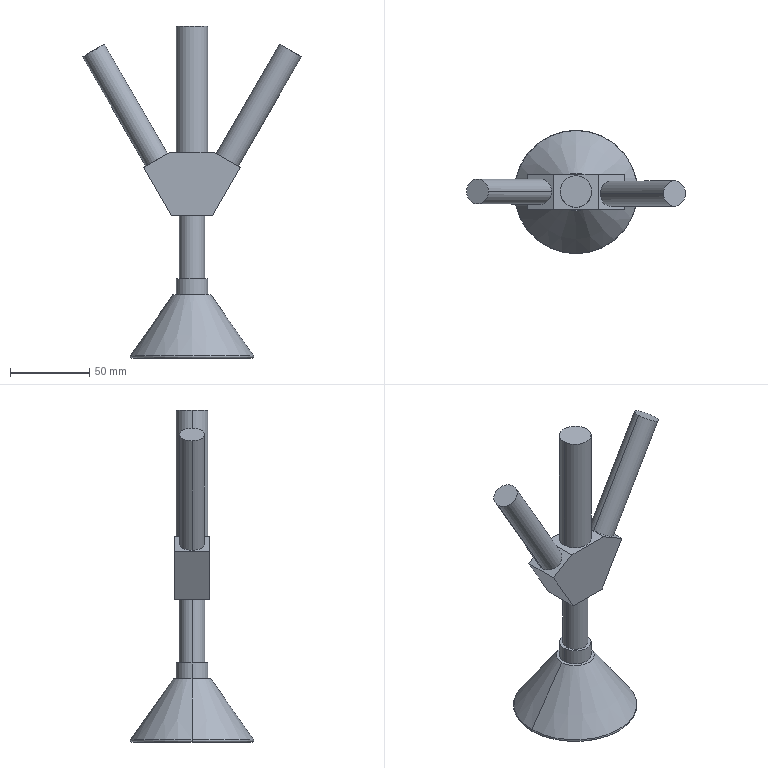Part | NX | features BREP 1 | 1 solid | 31 faces | box 138.349 x 78.158 x 210 mm | volume 141471 mm3 | plane 15 | cylinder 10 | cone 4 | torus 2 | commonest cylinder face diameters 16 x4 20 x4 15.837 x2
STEP:
#1=CARTESIAN_POINT('',(10.,0.,210.));
#2=VERTEX_POINT('',#1);
#3=CARTESIAN_POINT('',(-10.,0.,210.));
#4=VERTEX_POINT('',#3);
#5=CARTESIAN_POINT('',(0.,0.,210.));
#6=DIRECTION('',(0.,0.,1.));
#7=DIRECTION('',(1.,0.,0.));
#8=AXIS2_PLACEMENT_3D('',#5,#6,#7);
#9=CIRCLE('',#8,10.);
#10=EDGE_CURVE('',#2,#4,#9,.T.);
#11=ORIENTED_EDGE('',*,*,#10,.F.);
#12=CARTESIAN_POINT('',(10.,0.,130.));
#13=VERTEX_POINT('',#12);
#14=CARTESIAN_POINT('',(10.,0.,210.));
#15=DIRECTION('',(0.,0.,-1.));
#16=VECTOR('',#15,1000.);
#17=LINE('',#14,#16);
#18=EDGE_CURVE('',#2,#13,#17,.T.);
#19=ORIENTED_EDGE('',*,*,#18,.T.);
#20=CARTESIAN_POINT('',(-10.,0.,130.));
#21=VERTEX_POINT('',#20);
#22=CARTESIAN_POINT('',(0.,0.,130.));
#23=DIRECTION('',(0.,0.,1.));
#24=DIRECTION('',(1.,0.,0.));
#25=AXIS2_PLACEMENT_3D('',#22,#23,#24);
#26=CIRCLE('',#25,10.);
#27=EDGE_CURVE('',#13,#21,#26,.T.);
#28=ORIENTED_EDGE('',*,*,#27,.T.);
#29=CARTESIAN_POINT('',(-10.,0.,210.));
#30=DIRECTION('',(0.,0.,-1.));
#31=VECTOR('',#30,1000.);
#32=LINE('',#29,#31);
#33=EDGE_CURVE('',#4,#21,#32,.T.);
#34=ORIENTED_EDGE('',*,*,#33,.F.);
#35=EDGE_LOOP('',(#11,#19,#28,#34));
#36=FACE_BOUND('',#35,.T.);
#37=CARTESIAN_POINT('',(0.,0.,210.));
#38=DIRECTION('',(0.,0.,-1.));
#39=DIRECTION('',(-1.,0.,0.));
#40=AXIS2_PLACEMENT_3D('',#37,#38,#39);
#41=CYLINDRICAL_SURFACE('',#40,10.);
#42=ADVANCED_FACE('',(#36),#41,.T.);
#43=CARTESIAN_POINT('',(69.21,-1.268,190.503));
#44=VERTEX_POINT('',#43);
#45=CARTESIAN_POINT('',(55.353,-1.268,198.503));
#46=VERTEX_POINT('',#45);
#47=CARTESIAN_POINT('',(62.282,-1.268,194.503));
#48=DIRECTION('',(0.5,0.,0.866));
#49=DIRECTION('',(0.866,0.,-0.5));
#50=AXIS2_PLACEMENT_3D('',#47,#48,#49);
#51=CIRCLE('',#50,8.);
#52=EDGE_CURVE('',#44,#46,#51,.T.);
#53=ORIENTED_EDGE('',*,*,#52,.F.);
#54=CARTESIAN_POINT('',(29.21,-1.268,121.221));
#55=VERTEX_POINT('',#54);
#56=CARTESIAN_POINT('',(69.21,-1.268,190.503));
#57=DIRECTION('',(-0.5,0.,-0.866));
#58=VECTOR('',#57,1000.);
#59=LINE('',#56,#58);
#60=EDGE_CURVE('',#44,#55,#59,.T.);
#61=ORIENTED_EDGE('',*,*,#60,.T.);
#62=CARTESIAN_POINT('',(15.353,-1.268,129.221));
#63=VERTEX_POINT('',#62);
#64=CARTESIAN_POINT('',(22.282,-1.268,125.221));
#65=DIRECTION('',(0.5,0.,0.866));
#66=DIRECTION('',(0.866,0.,-0.5));
#67=AXIS2_PLACEMENT_3D('',#64,#65,#66);
#68=CIRCLE('',#67,8.);
#69=EDGE_CURVE('',#55,#63,#68,.T.);
#70=ORIENTED_EDGE('',*,*,#69,.T.);
#71=CARTESIAN_POINT('',(55.353,-1.268,198.503));
#72=DIRECTION('',(-0.5,0.,-0.866));
#73=VECTOR('',#72,1000.);
#74=LINE('',#71,#73);
#75=EDGE_CURVE('',#46,#63,#74,.T.);
#76=ORIENTED_EDGE('',*,*,#75,.F.);
#77=EDGE_LOOP('',(#53,#61,#70,#76));
#78=FACE_BOUND('',#77,.T.);
#79=CARTESIAN_POINT('',(62.282,-1.268,194.503));
#80=DIRECTION('',(-0.5,0.,-0.866));
#81=DIRECTION('',(-0.866,0.,0.5));
#82=AXIS2_PLACEMENT_3D('',#79,#80,#81);
#83=CYLINDRICAL_SURFACE('',#82,8.);
#84=ADVANCED_FACE('',(#78),#83,.T.);
#85=CARTESIAN_POINT('',(-55.424,0.,198.462));
#86=VERTEX_POINT('',#85);
#87=CARTESIAN_POINT('',(-69.139,0.,190.544));
#88=VERTEX_POINT('',#87);
#89=CARTESIAN_POINT('',(-62.282,0.,194.503));
#90=DIRECTION('',(-0.5,0.,0.866));
#91=DIRECTION('',(0.866,0.,0.5));
#92=AXIS2_PLACEMENT_3D('',#89,#90,#91);
#93=CIRCLE('',#92,7.918);
#94=EDGE_CURVE('',#86,#88,#93,.T.);
#95=ORIENTED_EDGE('',*,*,#94,.F.);
#96=CARTESIAN_POINT('',(-15.424,0.,129.18));
#97=VERTEX_POINT('',#96);
#98=CARTESIAN_POINT('',(-55.424,0.,198.462));
#99=DIRECTION('',(0.5,0.,-0.866));
#100=VECTOR('',#99,1000.);
#101=LINE('',#98,#100);
#102=EDGE_CURVE('',#86,#97,#101,.T.);
#103=ORIENTED_EDGE('',*,*,#102,.T.);
#104=CARTESIAN_POINT('',(-29.139,0.,121.262));
#105=VERTEX_POINT('',#104);
#106=CARTESIAN_POINT('',(-22.282,0.,125.221));
#107=DIRECTION('',(-0.5,0.,0.866));
#108=DIRECTION('',(0.866,0.,0.5));
#109=AXIS2_PLACEMENT_3D('',#106,#107,#108);
#110=CIRCLE('',#109,7.918);
#111=EDGE_CURVE('',#97,#105,#110,.T.);
#112=ORIENTED_EDGE('',*,*,#111,.T.);
#113=CARTESIAN_POINT('',(-69.139,0.,190.544));
#114=DIRECTION('',(0.5,0.,-0.866));
#115=VECTOR('',#114,1000.);
#116=LINE('',#113,#115);
#117=EDGE_CURVE('',#88,#105,#116,.T.);
#118=ORIENTED_EDGE('',*,*,#117,.F.);
#119=EDGE_LOOP('',(#95,#103,#112,#118));
#120=FACE_BOUND('',#119,.T.);
#121=CARTESIAN_POINT('',(-62.282,0.,194.503));
#122=DIRECTION('',(0.5,0.,-0.866));
#123=DIRECTION('',(-0.866,0.,-0.5));
#124=AXIS2_PLACEMENT_3D('',#121,#122,#123);
#125=CYLINDRICAL_SURFACE('',#124,7.918);
#126=ADVANCED_FACE('',(#120),#125,.T.);
#127=CARTESIAN_POINT('',(8.,0.,90.));
#128=VERTEX_POINT('',#127);
#129=CARTESIAN_POINT('',(-8.,0.,90.));
#130=VERTEX_POINT('',#129);
#131=CARTESIAN_POINT('',(0.,0.,90.));
#132=DIRECTION('',(0.,0.,1.));
#133=DIRECTION('',(1.,0.,0.));
#134=AXIS2_PLACEMENT_3D('',#131,#132,#133);
#135=CIRCLE('',#134,8.);
#136=EDGE_CURVE('',#128,#130,#135,.T.);
#137=ORIENTED_EDGE('',*,*,#136,.F.);
#138=CARTESIAN_POINT('',(8.,0.,50.));
#139=VERTEX_POINT('',#138);
#140=CARTESIAN_POINT('',(8.,0.,90.));
#141=DIRECTION('',(0.,0.,-1.));
#142=VECTOR('',#141,1000.);
#143=LINE('',#140,#142);
#144=EDGE_CURVE('',#128,#139,#143,.T.);
#145=ORIENTED_EDGE('',*,*,#144,.T.);
#146=CARTESIAN_POINT('',(-8.,0.,50.));
#147=VERTEX_POINT('',#146);
#148=CARTESIAN_POINT('',(0.,0.,50.));
#149=DIRECTION('',(0.,0.,1.));
#150=DIRECTION('',(1.,0.,0.));
#151=AXIS2_PLACEMENT_3D('',#148,#149,#150);
#152=CIRCLE('',#151,8.);
#153=EDGE_CURVE('',#139,#147,#152,.T.);
#154=ORIENTED_EDGE('',*,*,#153,.T.);
#155=CARTESIAN_POINT('',(-8.,0.,90.));
#156=DIRECTION('',(0.,0.,-1.));
#157=VECTOR('',#156,1000.);
#158=LINE('',#155,#157);
#159=EDGE_CURVE('',#130,#147,#158,.T.);
#160=ORIENTED_EDGE('',*,*,#159,.F.);
#161=EDGE_LOOP('',(#137,#145,#154,#160));
#162=FACE_BOUND('',#161,.T.);
#163=CARTESIAN_POINT('',(0.,0.,90.));
#164=DIRECTION('',(0.,0.,-1.));
#165=DIRECTION('',(-1.,0.,0.));
#166=AXIS2_PLACEMENT_3D('',#163,#164,#165);
#167=CYLINDRICAL_SURFACE('',#166,8.);
#168=ADVANCED_FACE('',(#162),#167,.T.);
#169=CARTESIAN_POINT('',(10.,0.,50.));
#170=VERTEX_POINT('',#169);
#171=CARTESIAN_POINT('',(-10.,0.,50.));
#172=VERTEX_POINT('',#171);
#173=CARTESIAN_POINT('',(0.,0.,50.));
#174=DIRECTION('',(0.,0.,1.));
#175=DIRECTION('',(1.,0.,0.));
#176=AXIS2_PLACEMENT_3D('',#173,#174,#175);
#177=CIRCLE('',#176,10.);
#178=EDGE_CURVE('',#170,#172,#177,.T.);
#179=ORIENTED_EDGE('',*,*,#178,.F.);
#180=CARTESIAN_POINT('',(10.,0.,40.));
#181=VERTEX_POINT('',#180);
#182=CARTESIAN_POINT('',(10.,0.,50.));
#183=DIRECTION('',(0.,0.,-1.));
#184=VECTOR('',#183,1000.);
#185=LINE('',#182,#184);
#186=EDGE_CURVE('',#170,#181,#185,.T.);
#187=ORIENTED_EDGE('',*,*,#186,.T.);
#188=CARTESIAN_POINT('',(-10.,0.,40.));
#189=VERTEX_POINT('',#188);
#190=CARTESIAN_POINT('',(0.,0.,40.));
#191=DIRECTION('',(0.,0.,1.));
#192=DIRECTION('',(1.,0.,0.));
#193=AXIS2_PLACEMENT_3D('',#190,#191,#192);
#194=CIRCLE('',#193,10.);
#195=EDGE_CURVE('',#181,#189,#194,.T.);
#196=ORIENTED_EDGE('',*,*,#195,.T.);
#197=CARTESIAN_POINT('',(-10.,0.,50.));
#198=DIRECTION('',(0.,0.,-1.));
#199=VECTOR('',#198,1000.);
#200=LINE('',#197,#199);
#201=EDGE_CURVE('',#172,#189,#200,.T.);
#202=ORIENTED_EDGE('',*,*,#201,.F.);
#203=EDGE_LOOP('',(#179,#187,#196,#202));
#204=FACE_BOUND('',#203,.T.);
#205=CARTESIAN_POINT('',(0.,0.,50.));
#206=DIRECTION('',(0.,0.,-1.));
#207=DIRECTION('',(-1.,0.,0.));
#208=AXIS2_PLACEMENT_3D('',#205,#206,#207);
#209=CYLINDRICAL_SURFACE('',#208,10.);
#210=ADVANCED_FACE('',(#204),#209,.T.);
#211=CARTESIAN_POINT('',(-38.079,0.,0.));
#212=VERTEX_POINT('',#211);
#213=CARTESIAN_POINT('',(38.079,0.,0.));
#214=VERTEX_POINT('',#213);
#215=CARTESIAN_POINT('',(0.,0.,0.));
#216=DIRECTION('',(0.,0.,-1.));
#217=DIRECTION('',(1.,0.,0.));
#218=AXIS2_PLACEMENT_3D('',#215,#216,#217);
#219=CIRCLE('',#218,38.079);
#220=EDGE_CURVE('',#212,#214,#219,.T.);
#221=ORIENTED_EDGE('',*,*,#220,.F.);
#222=CARTESIAN_POINT('',(-38.898,0.,1.574));
#223=VERTEX_POINT('',#222);
#224=CARTESIAN_POINT('',(-38.079,0.,1.));
#225=DIRECTION('',(0.,1.,0.));
#226=DIRECTION('',(-1.,0.,0.));
#227=AXIS2_PLACEMENT_3D('',#224,#225,#226);
#228=CIRCLE('',#227,1.);
#229=EDGE_CURVE('',#223,#212,#228,.F.);
#230=ORIENTED_EDGE('',*,*,#229,.F.);
#231=CARTESIAN_POINT('',(38.898,0.,1.574));
#232=VERTEX_POINT('',#231);
#233=CARTESIAN_POINT('',(0.,0.,1.574));
#234=DIRECTION('',(0.,0.,1.));
#235=DIRECTION('',(1.,0.,0.));
#236=AXIS2_PLACEMENT_3D('',#233,#234,#235);
#237=CIRCLE('',#236,38.898);
#238=EDGE_CURVE('',#232,#223,#237,.T.);
#239=ORIENTED_EDGE('',*,*,#238,.F.);
#240=CARTESIAN_POINT('',(38.079,0.,1.));
#241=DIRECTION('',(0.,-1.,0.));
#242=DIRECTION('',(0.,0.,-1.));
#243=AXIS2_PLACEMENT_3D('',#240,#241,#242);
#244=CIRCLE('',#243,1.);
#245=EDGE_CURVE('',#232,#214,#244,.F.);
#246=ORIENTED_EDGE('',*,*,#245,.T.);
#247=EDGE_LOOP('',(#221,#230,#239,#246));
#248=FACE_BOUND('',#247,.T.);
#249=CARTESIAN_POINT('',(0.,0.,1.));
#250=DIRECTION('',(0.,0.,1.));
#251=DIRECTION('',(1.,0.,0.));
#252=AXIS2_PLACEMENT_3D('',#249,#250,#251);
#253=TOROIDAL_SURFACE('',#252,38.079,1.);
#254=ADVANCED_FACE('',(#248),#253,.T.);
#255=CARTESIAN_POINT('',(5.992,0.,40.));
#256=VERTEX_POINT('',#255);
#257=CARTESIAN_POINT('',(-5.992,0.,40.));
#258=VERTEX_POINT('',#257);
#259=CARTESIAN_POINT('',(0.,0.,40.));
#260=DIRECTION('',(0.,0.,-1.));
#261=DIRECTION('',(-1.,0.,0.));
#262=AXIS2_PLACEMENT_3D('',#259,#260,#261);
#263=CIRCLE('',#262,5.992);
#264=EDGE_CURVE('',#256,#258,#263,.T.);
#265=ORIENTED_EDGE('',*,*,#264,.F.);
#266=CARTESIAN_POINT('',(34.,0.,0.));
#267=VERTEX_POINT('',#266);
#268=CARTESIAN_POINT('',(34.,0.,0.));
#269=DIRECTION('',(0.5736,0.,-0.8192));
#270=VECTOR('',#269,1000.);
#271=LINE('',#268,#270);
#272=EDGE_CURVE('',#256,#267,#271,.T.);
#273=ORIENTED_EDGE('',*,*,#272,.T.);
#274=CARTESIAN_POINT('',(-34.,0.,0.));
#275=VERTEX_POINT('',#274);
#276=CARTESIAN_POINT('',(0.,0.,0.));
#277=DIRECTION('',(0.,0.,-1.));
#278=DIRECTION('',(-1.,0.,0.));
#279=AXIS2_PLACEMENT_3D('',#276,#277,#278);
#280=CIRCLE('',#279,34.);
#281=EDGE_CURVE('',#267,#275,#280,.T.);
#282=ORIENTED_EDGE('',*,*,#281,.T.);
#283=CARTESIAN_POINT('',(-34.,0.,0.));
#284=DIRECTION('',(-0.5736,0.,-0.8192));
#285=VECTOR('',#284,1000.);
#286=LINE('',#283,#285);
#287=EDGE_CURVE('',#258,#275,#286,.T.);
#288=ORIENTED_EDGE('',*,*,#287,.F.);
#289=EDGE_LOOP('',(#265,#273,#282,#288));
#290=FACE_BOUND('',#289,.T.);
#291=CARTESIAN_POINT('',(0.,0.,0.));
#292=DIRECTION('',(0.,0.,-1.));
#293=DIRECTION('',(-1.,0.,0.));
#294=AXIS2_PLACEMENT_3D('',#291,#292,#293);
#295=CONICAL_SURFACE('',#294,34.,0.6109);
#296=ADVANCED_FACE('',(#290),#295,.F.);
#297=CARTESIAN_POINT('',(-11.992,0.,40.));
#298=VERTEX_POINT('',#297);
#299=CARTESIAN_POINT('',(11.992,0.,40.));
#300=VERTEX_POINT('',#299);
#301=CARTESIAN_POINT('',(0.,0.,40.));
#302=DIRECTION('',(0.,0.,1.));
#303=DIRECTION('',(1.,0.,0.));
#304=AXIS2_PLACEMENT_3D('',#301,#302,#303);
#305=CIRCLE('',#304,11.992);
#306=EDGE_CURVE('',#298,#300,#305,.T.);
#307=ORIENTED_EDGE('',*,*,#306,.F.);
#308=CARTESIAN_POINT('',(-40.,0.,0.));
#309=DIRECTION('',(-0.5736,0.,-0.8192));
#310=VECTOR('',#309,1000.);
#311=LINE('',#308,#310);
#312=EDGE_CURVE('',#223,#298,#311,.F.);
#313=ORIENTED_EDGE('',*,*,#312,.F.);
#314=CARTESIAN_POINT('',(0.,0.,1.574));
#315=DIRECTION('',(0.,0.,1.));
#316=DIRECTION('',(1.,0.,0.));
#317=AXIS2_PLACEMENT_3D('',#314,#315,#316);
#318=CIRCLE('',#317,38.898);
#319=EDGE_CURVE('',#223,#232,#318,.T.);
#320=ORIENTED_EDGE('',*,*,#319,.T.);
#321=CARTESIAN_POINT('',(40.,0.,0.));
#322=DIRECTION('',(0.5736,0.,-0.8192));
#323=VECTOR('',#322,1000.);
#324=LINE('',#321,#323);
#325=EDGE_CURVE('',#232,#300,#324,.F.);
#326=ORIENTED_EDGE('',*,*,#325,.T.);
#327=EDGE_LOOP('',(#307,#313,#320,#326));
#328=FACE_BOUND('',#327,.T.);
#329=CARTESIAN_POINT('',(0.,0.,0.));
#330=DIRECTION('',(0.,0.,-1.));
#331=DIRECTION('',(1.,0.,0.));
#332=AXIS2_PLACEMENT_3D('',#329,#330,#331);
#333=CONICAL_SURFACE('',#332,40.,0.6109);
#334=ADVANCED_FACE('',(#328),#333,.T.);
#335=ORIENTED_EDGE('',*,*,#312,.T.);
#336=CARTESIAN_POINT('',(0.,0.,40.));
#337=DIRECTION('',(0.,0.,1.));
#338=DIRECTION('',(1.,0.,0.));
#339=AXIS2_PLACEMENT_3D('',#336,#337,#338);
#340=CIRCLE('',#339,11.992);
#341=EDGE_CURVE('',#300,#298,#340,.T.);
#342=ORIENTED_EDGE('',*,*,#341,.F.);
#343=ORIENTED_EDGE('',*,*,#325,.F.);
#344=ORIENTED_EDGE('',*,*,#238,.T.);
#345=EDGE_LOOP('',(#335,#342,#343,#344));
#346=FACE_BOUND('',#345,.T.);
#347=CARTESIAN_POINT('',(0.,0.,0.));
#348=DIRECTION('',(0.,0.,-1.));
#349=DIRECTION('',(1.,0.,0.));
#350=AXIS2_PLACEMENT_3D('',#347,#348,#349);
#351=CONICAL_SURFACE('',#350,40.,0.6109);
#352=ADVANCED_FACE('',(#346),#351,.T.);
#353=ORIENTED_EDGE('',*,*,#341,.T.);
#354=ORIENTED_EDGE('',*,*,#306,.T.);
#355=EDGE_LOOP('',(#353,#354));
#356=FACE_BOUND('',#355,.T.);
#357=CARTESIAN_POINT('',(0.,0.,40.));
#358=DIRECTION('',(0.,0.,1.));
#359=DIRECTION('',(1.,0.,0.));
#360=AXIS2_PLACEMENT_3D('',#357,#358,#359);
#361=CIRCLE('',#360,10.);
#362=EDGE_CURVE('',#189,#181,#361,.T.);
#363=ORIENTED_EDGE('',*,*,#362,.F.);
#364=ORIENTED_EDGE('',*,*,#195,.F.);
#365=EDGE_LOOP('',(#363,#364));
#366=FACE_BOUND('',#365,.T.);
#367=CARTESIAN_POINT('',(0.,0.,40.));
#368=DIRECTION('',(0.,0.,1.));
#369=DIRECTION('',(1.,0.,0.));
#370=AXIS2_PLACEMENT_3D('',#367,#368,#369);
#371=PLANE('',#370);
#372=ADVANCED_FACE('',(#356,#366),#371,.T.);
#373=CARTESIAN_POINT('',(0.,0.,0.));
#374=DIRECTION('',(0.,0.,-1.));
#375=DIRECTION('',(1.,0.,0.));
#376=AXIS2_PLACEMENT_3D('',#373,#374,#375);
#377=CIRCLE('',#376,38.079);
#378=EDGE_CURVE('',#214,#212,#377,.T.);
#379=ORIENTED_EDGE('',*,*,#378,.T.);
#380=ORIENTED_EDGE('',*,*,#220,.T.);
#381=EDGE_LOOP('',(#379,#380));
#382=FACE_BOUND('',#381,.T.);
#383=CARTESIAN_POINT('',(0.,0.,0.));
#384=DIRECTION('',(0.,0.,-1.));
#385=DIRECTION('',(-1.,0.,0.));
#386=AXIS2_PLACEMENT_3D('',#383,#384,#385);
#387=CIRCLE('',#386,34.);
#388=EDGE_CURVE('',#275,#267,#387,.T.);
#389=ORIENTED_EDGE('',*,*,#388,.F.);
#390=ORIENTED_EDGE('',*,*,#281,.F.);
#391=EDGE_LOOP('',(#389,#390));
#392=FACE_BOUND('',#391,.T.);
#393=CARTESIAN_POINT('',(0.,0.,0.));
#394=DIRECTION('',(0.,0.,1.));
#395=DIRECTION('',(1.,0.,0.));
#396=AXIS2_PLACEMENT_3D('',#393,#394,#395);
#397=PLANE('',#396);
#398=ADVANCED_FACE('',(#382,#392),#397,.F.);
#399=ORIENTED_EDGE('',*,*,#272,.F.);
#400=CARTESIAN_POINT('',(0.,0.,40.));
#401=DIRECTION('',(0.,0.,-1.));
#402=DIRECTION('',(-1.,0.,0.));
#403=AXIS2_PLACEMENT_3D('',#400,#401,#402);
#404=CIRCLE('',#403,5.992);
#405=EDGE_CURVE('',#258,#256,#404,.T.);
#406=ORIENTED_EDGE('',*,*,#405,.F.);
#407=ORIENTED_EDGE('',*,*,#287,.T.);
#408=ORIENTED_EDGE('',*,*,#388,.T.);
#409=EDGE_LOOP('',(#399,#406,#407,#408));
#410=FACE_BOUND('',#409,.T.);
#411=CARTESIAN_POINT('',(0.,0.,0.));
#412=DIRECTION('',(0.,0.,-1.));
#413=DIRECTION('',(-1.,0.,0.));
#414=AXIS2_PLACEMENT_3D('',#411,#412,#413);
#415=CONICAL_SURFACE('',#414,34.,0.6109);
#416=ADVANCED_FACE('',(#410),#415,.F.);
#417=ORIENTED_EDGE('',*,*,#229,.T.);
#418=ORIENTED_EDGE('',*,*,#378,.F.);
#419=ORIENTED_EDGE('',*,*,#245,.F.);
#420=ORIENTED_EDGE('',*,*,#319,.F.);
#421=EDGE_LOOP('',(#417,#418,#419,#420));
#422=FACE_BOUND('',#421,.T.);
#423=CARTESIAN_POINT('',(0.,0.,1.));
#424=DIRECTION('',(0.,0.,1.));
#425=DIRECTION('',(1.,0.,0.));
#426=AXIS2_PLACEMENT_3D('',#423,#424,#425);
#427=TOROIDAL_SURFACE('',#426,38.079,1.);
#428=ADVANCED_FACE('',(#422),#427,.T.);
#429=CARTESIAN_POINT('',(0.,0.,50.));
#430=DIRECTION('',(0.,0.,1.));
#431=DIRECTION('',(1.,0.,0.));
#432=AXIS2_PLACEMENT_3D('',#429,#430,#431);
#433=CIRCLE('',#432,10.);
#434=EDGE_CURVE('',#172,#170,#433,.T.);
#435=ORIENTED_EDGE('',*,*,#434,.T.);
#436=ORIENTED_EDGE('',*,*,#178,.T.);
#437=EDGE_LOOP('',(#435,#436));
#438=FACE_BOUND('',#437,.T.);
#439=CARTESIAN_POINT('',(0.,0.,50.));
#440=DIRECTION('',(0.,0.,1.));
#441=DIRECTION('',(1.,0.,0.));
#442=AXIS2_PLACEMENT_3D('',#439,#440,#441);
#443=CIRCLE('',#442,8.);
#444=EDGE_CURVE('',#147,#139,#443,.T.);
#445=ORIENTED_EDGE('',*,*,#444,.F.);
#446=ORIENTED_EDGE('',*,*,#153,.F.);
#447=EDGE_LOOP('',(#445,#446));
#448=FACE_BOUND('',#447,.T.);
#449=CARTESIAN_POINT('',(0.,0.,50.));
#450=DIRECTION('',(0.,0.,1.));
#451=DIRECTION('',(1.,0.,0.));
#452=AXIS2_PLACEMENT_3D('',#449,#450,#451);
#453=PLANE('',#452);
#454=ADVANCED_FACE('',(#438,#448),#453,.T.);
#455=ORIENTED_EDGE('',*,*,#186,.F.);
#456=ORIENTED_EDGE('',*,*,#434,.F.);
#457=ORIENTED_EDGE('',*,*,#201,.T.);
#458=ORIENTED_EDGE('',*,*,#362,.T.);
#459=EDGE_LOOP('',(#455,#456,#457,#458));
#460=FACE_BOUND('',#459,.T.);
#461=CARTESIAN_POINT('',(0.,0.,50.));
#462=DIRECTION('',(0.,0.,-1.));
#463=DIRECTION('',(-1.,0.,0.));
#464=AXIS2_PLACEMENT_3D('',#461,#462,#463);
#465=CYLINDRICAL_SURFACE('',#464,10.);
#466=ADVANCED_FACE('',(#460),#465,.T.);
#467=ORIENTED_EDGE('',*,*,#405,.T.);
#468=ORIENTED_EDGE('',*,*,#264,.T.);
#469=EDGE_LOOP('',(#467,#468));
#470=FACE_BOUND('',#469,.T.);
#471=CARTESIAN_POINT('',(0.,0.,40.));
#472=DIRECTION('',(0.,0.,1.));
#473=DIRECTION('',(1.,0.,0.));
#474=AXIS2_PLACEMENT_3D('',#471,#472,#473);
#475=PLANE('',#474);
#476=ADVANCED_FACE('',(#470),#475,.F.);
#477=ORIENTED_EDGE('',*,*,#144,.F.);
#478=CARTESIAN_POINT('',(0.,0.,90.));
#479=DIRECTION('',(0.,0.,1.));
#480=DIRECTION('',(1.,0.,0.));
#481=AXIS2_PLACEMENT_3D('',#478,#479,#480);
#482=CIRCLE('',#481,8.);
#483=EDGE_CURVE('',#130,#128,#482,.T.);
#484=ORIENTED_EDGE('',*,*,#483,.F.);
#485=ORIENTED_EDGE('',*,*,#159,.T.);
#486=ORIENTED_EDGE('',*,*,#444,.T.);
#487=EDGE_LOOP('',(#477,#484,#485,#486));
#488=FACE_BOUND('',#487,.T.);
#489=CARTESIAN_POINT('',(0.,0.,90.));
#490=DIRECTION('',(0.,0.,-1.));
#491=DIRECTION('',(-1.,0.,0.));
#492=AXIS2_PLACEMENT_3D('',#489,#490,#491);
#493=CYLINDRICAL_SURFACE('',#492,8.);
#494=ADVANCED_FACE('',(#488),#493,.T.);
#495=CARTESIAN_POINT('',(12.983,11.088,90.));
#496=VERTEX_POINT('',#495);
#497=CARTESIAN_POINT('',(-12.983,11.088,90.));
#498=VERTEX_POINT('',#497);
#499=CARTESIAN_POINT('',(-12.983,11.088,90.));
#500=DIRECTION('',(-1.,0.,0.));
#501=VECTOR('',#500,1000.);
#502=LINE('',#499,#501);
#503=EDGE_CURVE('',#496,#498,#502,.T.);
#504=ORIENTED_EDGE('',*,*,#503,.T.);
#505=CARTESIAN_POINT('',(-30.559,11.088,120.442));
#506=VERTEX_POINT('',#505);
#507=CARTESIAN_POINT('',(-12.983,11.088,90.));
#508=DIRECTION('',(-0.5,0.,0.866));
#509=VECTOR('',#508,1000.);
#510=LINE('',#507,#509);
#511=EDGE_CURVE('',#498,#506,#510,.T.);
#512=ORIENTED_EDGE('',*,*,#511,.T.);
#513=CARTESIAN_POINT('',(-14.004,11.088,130.));
#514=VERTEX_POINT('',#513);
#515=CARTESIAN_POINT('',(-30.559,11.088,120.442));
#516=DIRECTION('',(0.866,0.,0.5));
#517=VECTOR('',#516,1000.);
#518=LINE('',#515,#517);
#519=EDGE_CURVE('',#506,#514,#518,.T.);
#520=ORIENTED_EDGE('',*,*,#519,.T.);
#521=CARTESIAN_POINT('',(14.004,11.088,130.));
#522=VERTEX_POINT('',#521);
#523=CARTESIAN_POINT('',(-12.983,11.088,130.));
#524=DIRECTION('',(-1.,0.,0.));
#525=VECTOR('',#524,1000.);
#526=LINE('',#523,#525);
#527=EDGE_CURVE('',#522,#514,#526,.T.);
#528=ORIENTED_EDGE('',*,*,#527,.F.);
#529=CARTESIAN_POINT('',(30.559,11.088,120.442));
#530=VERTEX_POINT('',#529);
#531=CARTESIAN_POINT('',(30.559,11.088,120.442));
#532=DIRECTION('',(0.866,0.,-0.5));
#533=VECTOR('',#532,1000.);
#534=LINE('',#531,#533);
#535=EDGE_CURVE('',#522,#530,#534,.T.);
#536=ORIENTED_EDGE('',*,*,#535,.T.);
#537=CARTESIAN_POINT('',(12.983,11.088,90.));
#538=DIRECTION('',(-0.5,0.,-0.866));
#539=VECTOR('',#538,1000.);
#540=LINE('',#537,#539);
#541=EDGE_CURVE('',#530,#496,#540,.T.);
#542=ORIENTED_EDGE('',*,*,#541,.T.);
#543=EDGE_LOOP('',(#504,#512,#520,#528,#536,#542));
#544=FACE_BOUND('',#543,.T.);
#545=CARTESIAN_POINT('',(-12.983,11.088,130.));
#546=DIRECTION('',(0.,-1.,0.));
#547=DIRECTION('',(0.,0.,-1.));
#548=AXIS2_PLACEMENT_3D('',#545,#546,#547);
#549=PLANE('',#548);
#550=ADVANCED_FACE('',(#544),#549,.F.);
#551=CARTESIAN_POINT('',(-12.983,-11.088,90.));
#552=VERTEX_POINT('',#551);
#553=CARTESIAN_POINT('',(12.983,-11.088,90.));
#554=VERTEX_POINT('',#553);
#555=CARTESIAN_POINT('',(-12.983,-11.088,90.));
#556=DIRECTION('',(1.,0.,0.));
#557=VECTOR('',#556,1000.);
#558=LINE('',#555,#557);
#559=EDGE_CURVE('',#552,#554,#558,.T.);
#560=ORIENTED_EDGE('',*,*,#559,.T.);
#561=CARTESIAN_POINT('',(30.559,-11.088,120.442));
#562=VERTEX_POINT('',#561);
#563=CARTESIAN_POINT('',(12.983,-11.088,90.));
#564=DIRECTION('',(0.5,0.,0.866));
#565=VECTOR('',#564,1000.);
#566=LINE('',#563,#565);
#567=EDGE_CURVE('',#554,#562,#566,.T.);
#568=ORIENTED_EDGE('',*,*,#567,.T.);
#569=CARTESIAN_POINT('',(14.004,-11.088,130.));
#570=VERTEX_POINT('',#569);
#571=CARTESIAN_POINT('',(30.559,-11.088,120.442));
#572=DIRECTION('',(-0.866,0.,0.5));
#573=VECTOR('',#572,1000.);
#574=LINE('',#571,#573);
#575=EDGE_CURVE('',#562,#570,#574,.T.);
#576=ORIENTED_EDGE('',*,*,#575,.T.);
#577=CARTESIAN_POINT('',(-14.004,-11.088,130.));
#578=VERTEX_POINT('',#577);
#579=CARTESIAN_POINT('',(-12.983,-11.088,130.));
#580=DIRECTION('',(1.,0.,0.));
#581=VECTOR('',#580,1000.);
#582=LINE('',#579,#581);
#583=EDGE_CURVE('',#578,#570,#582,.T.);
#584=ORIENTED_EDGE('',*,*,#583,.F.);
#585=CARTESIAN_POINT('',(-30.559,-11.088,120.442));
#586=VERTEX_POINT('',#585);
#587=CARTESIAN_POINT('',(-30.559,-11.088,120.442));
#588=DIRECTION('',(-0.866,0.,-0.5));
#589=VECTOR('',#588,1000.);
#590=LINE('',#587,#589);
#591=EDGE_CURVE('',#578,#586,#590,.T.);
#592=ORIENTED_EDGE('',*,*,#591,.T.);
#593=CARTESIAN_POINT('',(-12.983,-11.088,90.));
#594=DIRECTION('',(0.5,0.,-0.866));
#595=VECTOR('',#594,1000.);
#596=LINE('',#593,#595);
#597=EDGE_CURVE('',#586,#552,#596,.T.);
#598=ORIENTED_EDGE('',*,*,#597,.T.);
#599=EDGE_LOOP('',(#560,#568,#576,#584,#592,#598));
#600=FACE_BOUND('',#599,.T.);
#601=CARTESIAN_POINT('',(-12.983,-11.088,130.));
#602=DIRECTION('',(0.,1.,0.));
#603=DIRECTION('',(1.,0.,0.));
#604=AXIS2_PLACEMENT_3D('',#601,#602,#603);
#605=PLANE('',#604);
#606=ADVANCED_FACE('',(#600),#605,.F.);
#607=ORIENTED_EDGE('',*,*,#583,.T.);
#608=CARTESIAN_POINT('',(14.004,-54.779,130.));
#609=DIRECTION('',(0.,1.,0.));
#610=VECTOR('',#609,1000.);
#611=LINE('',#608,#610);
#612=EDGE_CURVE('',#570,#522,#611,.T.);
#613=ORIENTED_EDGE('',*,*,#612,.T.);
#614=ORIENTED_EDGE('',*,*,#527,.T.);
#615=CARTESIAN_POINT('',(-14.004,-54.779,130.));
#616=DIRECTION('',(0.,1.,0.));
#617=VECTOR('',#616,1000.);
#618=LINE('',#615,#617);
#619=EDGE_CURVE('',#578,#514,#618,.T.);
#620=ORIENTED_EDGE('',*,*,#619,.F.);
#621=EDGE_LOOP('',(#607,#613,#614,#620));
#622=FACE_BOUND('',#621,.T.);
#623=CARTESIAN_POINT('',(0.,0.,130.));
#624=DIRECTION('',(0.,0.,1.));
#625=DIRECTION('',(1.,0.,0.));
#626=AXIS2_PLACEMENT_3D('',#623,#624,#625);
#627=CIRCLE('',#626,10.);
#628=EDGE_CURVE('',#21,#13,#627,.T.);
#629=ORIENTED_EDGE('',*,*,#628,.F.);
#630=ORIENTED_EDGE('',*,*,#27,.F.);
#631=EDGE_LOOP('',(#629,#630));
#632=FACE_BOUND('',#631,.T.);
#633=CARTESIAN_POINT('',(0.,0.,130.));
#634=DIRECTION('',(0.,0.,-1.));
#635=DIRECTION('',(0.,-1.,0.));
#636=AXIS2_PLACEMENT_3D('',#633,#634,#635);
#637=PLANE('',#636);
#638=ADVANCED_FACE('',(#622,#632),#637,.F.);
#639=CARTESIAN_POINT('',(12.983,-11.088,90.));
#640=DIRECTION('',(0.,1.,0.));
#641=VECTOR('',#640,1000.);
#642=LINE('',#639,#641);
#643=EDGE_CURVE('',#554,#496,#642,.T.);
#644=ORIENTED_EDGE('',*,*,#643,.F.);
#645=ORIENTED_EDGE('',*,*,#559,.F.);
#646=CARTESIAN_POINT('',(-12.983,-11.088,90.));
#647=DIRECTION('',(0.,-1.,0.));
#648=VECTOR('',#647,1000.);
#649=LINE('',#646,#648);
#650=EDGE_CURVE('',#498,#552,#649,.T.);
#651=ORIENTED_EDGE('',*,*,#650,.F.);
#652=ORIENTED_EDGE('',*,*,#503,.F.);
#653=EDGE_LOOP('',(#644,#645,#651,#652));
#654=FACE_BOUND('',#653,.T.);
#655=ORIENTED_EDGE('',*,*,#483,.T.);
#656=ORIENTED_EDGE('',*,*,#136,.T.);
#657=EDGE_LOOP('',(#655,#656));
#658=FACE_BOUND('',#657,.T.);
#659=CARTESIAN_POINT('',(0.,0.,90.));
#660=DIRECTION('',(0.,0.,-1.));
#661=DIRECTION('',(0.,-1.,0.));
#662=AXIS2_PLACEMENT_3D('',#659,#660,#661);
#663=PLANE('',#662);
#664=ADVANCED_FACE('',(#654,#658),#663,.T.);
#665=ORIENTED_EDGE('',*,*,#591,.F.);
#666=ORIENTED_EDGE('',*,*,#619,.T.);
#667=ORIENTED_EDGE('',*,*,#519,.F.);
#668=CARTESIAN_POINT('',(-30.559,-54.779,120.442));
#669=DIRECTION('',(0.,1.,0.));
#670=VECTOR('',#669,1000.);
#671=LINE('',#668,#670);
#672=EDGE_CURVE('',#586,#506,#671,.T.);
#673=ORIENTED_EDGE('',*,*,#672,.F.);
#674=EDGE_LOOP('',(#665,#666,#667,#673));
#675=FACE_BOUND('',#674,.T.);
#676=CARTESIAN_POINT('',(-22.282,0.,125.221));
#677=DIRECTION('',(-0.5,0.,0.866));
#678=DIRECTION('',(0.866,0.,0.5));
#679=AXIS2_PLACEMENT_3D('',#676,#677,#678);
#680=CIRCLE('',#679,7.918);
#681=EDGE_CURVE('',#105,#97,#680,.T.);
#682=ORIENTED_EDGE('',*,*,#681,.F.);
#683=ORIENTED_EDGE('',*,*,#111,.F.);
#684=EDGE_LOOP('',(#682,#683));
#685=FACE_BOUND('',#684,.T.);
#686=CARTESIAN_POINT('',(-30.559,-54.779,120.442));
#687=DIRECTION('',(-0.5,0.,0.866));
#688=DIRECTION('',(0.,1.,0.));
#689=AXIS2_PLACEMENT_3D('',#686,#687,#688);
#690=PLANE('',#689);
#691=ADVANCED_FACE('',(#675,#685),#690,.T.);
#692=ORIENTED_EDGE('',*,*,#597,.F.);
#693=ORIENTED_EDGE('',*,*,#672,.T.);
#694=ORIENTED_EDGE('',*,*,#511,.F.);
#695=ORIENTED_EDGE('',*,*,#650,.T.);
#696=EDGE_LOOP('',(#692,#693,#694,#695));
#697=FACE_BOUND('',#696,.T.);
#698=CARTESIAN_POINT('',(-12.983,-54.779,90.));
#699=DIRECTION('',(-0.866,0.,-0.5));
#700=DIRECTION('',(-0.5,0.,0.866));
#701=AXIS2_PLACEMENT_3D('',#698,#699,#700);
#702=PLANE('',#701);
#703=ADVANCED_FACE('',(#697),#702,.T.);
#704=ORIENTED_EDGE('',*,*,#567,.F.);
#705=ORIENTED_EDGE('',*,*,#643,.T.);
#706=ORIENTED_EDGE('',*,*,#541,.F.);
#707=CARTESIAN_POINT('',(30.559,-54.779,120.442));
#708=DIRECTION('',(0.,1.,0.));
#709=VECTOR('',#708,1000.);
#710=LINE('',#707,#709);
#711=EDGE_CURVE('',#562,#530,#710,.T.);
#712=ORIENTED_EDGE('',*,*,#711,.F.);
#713=EDGE_LOOP('',(#704,#705,#706,#712));
#714=FACE_BOUND('',#713,.T.);
#715=CARTESIAN_POINT('',(12.983,-54.779,90.));
#716=DIRECTION('',(0.866,0.,-0.5));
#717=DIRECTION('',(0.,-1.,0.));
#718=AXIS2_PLACEMENT_3D('',#715,#716,#717);
#719=PLANE('',#718);
#720=ADVANCED_FACE('',(#714),#719,.T.);
#721=ORIENTED_EDGE('',*,*,#575,.F.);
#722=ORIENTED_EDGE('',*,*,#711,.T.);
#723=ORIENTED_EDGE('',*,*,#535,.F.);
#724=ORIENTED_EDGE('',*,*,#612,.F.);
#725=EDGE_LOOP('',(#721,#722,#723,#724));
#726=FACE_BOUND('',#725,.T.);
#727=CARTESIAN_POINT('',(22.282,-1.268,125.221));
#728=DIRECTION('',(0.5,0.,0.866));
#729=DIRECTION('',(0.866,0.,-0.5));
#730=AXIS2_PLACEMENT_3D('',#727,#728,#729);
#731=CIRCLE('',#730,8.);
#732=EDGE_CURVE('',#63,#55,#731,.T.);
#733=ORIENTED_EDGE('',*,*,#732,.F.);
#734=ORIENTED_EDGE('',*,*,#69,.F.);
#735=EDGE_LOOP('',(#733,#734));
#736=FACE_BOUND('',#735,.T.);
#737=CARTESIAN_POINT('',(30.559,-54.779,120.442));
#738=DIRECTION('',(0.5,0.,0.866));
#739=DIRECTION('',(0.,-1.,0.));
#740=AXIS2_PLACEMENT_3D('',#737,#738,#739);
#741=PLANE('',#740);
#742=ADVANCED_FACE('',(#726,#736),#741,.T.);
#743=ORIENTED_EDGE('',*,*,#102,.F.);
#744=CARTESIAN_POINT('',(-62.282,0.,194.503));
#745=DIRECTION('',(-0.5,0.,0.866));
#746=DIRECTION('',(0.866,0.,0.5));
#747=AXIS2_PLACEMENT_3D('',#744,#745,#746);
#748=CIRCLE('',#747,7.918);
#749=EDGE_CURVE('',#88,#86,#748,.T.);
#750=ORIENTED_EDGE('',*,*,#749,.F.);
#751=ORIENTED_EDGE('',*,*,#117,.T.);
#752=ORIENTED_EDGE('',*,*,#681,.T.);
#753=EDGE_LOOP('',(#743,#750,#751,#752));
#754=FACE_BOUND('',#753,.T.);
#755=CARTESIAN_POINT('',(-62.282,0.,194.503));
#756=DIRECTION('',(0.5,0.,-0.866));
#757=DIRECTION('',(-0.866,0.,-0.5));
#758=AXIS2_PLACEMENT_3D('',#755,#756,#757);
#759=CYLINDRICAL_SURFACE('',#758,7.918);
#760=ADVANCED_FACE('',(#754),#759,.T.);
#761=ORIENTED_EDGE('',*,*,#749,.T.);
#762=ORIENTED_EDGE('',*,*,#94,.T.);
#763=EDGE_LOOP('',(#761,#762));
#764=FACE_BOUND('',#763,.T.);
#765=CARTESIAN_POINT('',(-62.282,0.,194.503));
#766=DIRECTION('',(-0.5,0.,0.866));
#767=DIRECTION('',(0.,1.,0.));
#768=AXIS2_PLACEMENT_3D('',#765,#766,#767);
#769=PLANE('',#768);
#770=ADVANCED_FACE('',(#764),#769,.T.);
#771=ORIENTED_EDGE('',*,*,#60,.F.);
#772=CARTESIAN_POINT('',(62.282,-1.268,194.503));
#773=DIRECTION('',(0.5,0.,0.866));
#774=DIRECTION('',(0.866,0.,-0.5));
#775=AXIS2_PLACEMENT_3D('',#772,#773,#774);
#776=CIRCLE('',#775,8.);
#777=EDGE_CURVE('',#46,#44,#776,.T.);
#778=ORIENTED_EDGE('',*,*,#777,.F.);
#779=ORIENTED_EDGE('',*,*,#75,.T.);
#780=ORIENTED_EDGE('',*,*,#732,.T.);
#781=EDGE_LOOP('',(#771,#778,#779,#780));
#782=FACE_BOUND('',#781,.T.);
#783=CARTESIAN_POINT('',(62.282,-1.268,194.503));
#784=DIRECTION('',(-0.5,0.,-0.866));
#785=DIRECTION('',(-0.866,0.,0.5));
#786=AXIS2_PLACEMENT_3D('',#783,#784,#785);
#787=CYLINDRICAL_SURFACE('',#786,8.);
#788=ADVANCED_FACE('',(#782),#787,.T.);
#789=ORIENTED_EDGE('',*,*,#777,.T.);
#790=ORIENTED_EDGE('',*,*,#52,.T.);
#791=EDGE_LOOP('',(#789,#790));
#792=FACE_BOUND('',#791,.T.);
#793=CARTESIAN_POINT('',(62.282,-1.268,194.503));
#794=DIRECTION('',(0.5,0.,0.866));
#795=DIRECTION('',(0.,-1.,0.));
#796=AXIS2_PLACEMENT_3D('',#793,#794,#795);
#797=PLANE('',#796);
#798=ADVANCED_FACE('',(#792),#797,.T.);
#799=ORIENTED_EDGE('',*,*,#18,.F.);
#800=CARTESIAN_POINT('',(0.,0.,210.));
#801=DIRECTION('',(0.,0.,1.));
#802=DIRECTION('',(1.,0.,0.));
#803=AXIS2_PLACEMENT_3D('',#800,#801,#802);
#804=CIRCLE('',#803,10.);
#805=EDGE_CURVE('',#4,#2,#804,.T.);
#806=ORIENTED_EDGE('',*,*,#805,.F.);
#807=ORIENTED_EDGE('',*,*,#33,.T.);
#808=ORIENTED_EDGE('',*,*,#628,.T.);
#809=EDGE_LOOP('',(#799,#806,#807,#808));
#810=FACE_BOUND('',#809,.T.);
#811=CARTESIAN_POINT('',(0.,0.,210.));
#812=DIRECTION('',(0.,0.,-1.));
#813=DIRECTION('',(-1.,0.,0.));
#814=AXIS2_PLACEMENT_3D('',#811,#812,#813);
#815=CYLINDRICAL_SURFACE('',#814,10.);
#816=ADVANCED_FACE('',(#810),#815,.T.);
#817=ORIENTED_EDGE('',*,*,#805,.T.);
#818=ORIENTED_EDGE('',*,*,#10,.T.);
#819=EDGE_LOOP('',(#817,#818));
#820=FACE_BOUND('',#819,.T.);
#821=CARTESIAN_POINT('',(0.,0.,210.));
#822=DIRECTION('',(0.,0.,1.));
#823=DIRECTION('',(1.,0.,0.));
#824=AXIS2_PLACEMENT_3D('',#821,#822,#823);
#825=PLANE('',#824);
#826=ADVANCED_FACE('',(#820),#825,.T.);
#827=CLOSED_SHELL('',(#42,#84,#126,#168,#210,#254,#296,#334,#352,#372,#398,#416,#428,#454,#466,#476,#494,#550,#606,#638,#664,#691,#703,#720,#742,#760,#770,#788,#798,#816,#826));
#828=MANIFOLD_SOLID_BREP('',#827);
#829=(LENGTH_UNIT()NAMED_UNIT(*)SI_UNIT(.MILLI.,.METRE.));
#830=UNCERTAINTY_MEASURE_WITH_UNIT(LENGTH_MEASURE(0.00001),#829,'','');
#831=(NAMED_UNIT(*)PLANE_ANGLE_UNIT()SI_UNIT($,.RADIAN.));
#832=(NAMED_UNIT(*)SI_UNIT($,.STERADIAN.)SOLID_ANGLE_UNIT());
#833=(GEOMETRIC_REPRESENTATION_CONTEXT(3)GLOBAL_UNCERTAINTY_ASSIGNED_CONTEXT((#830))GLOBAL_UNIT_ASSIGNED_CONTEXT((#829,#831,#832))REPRESENTATION_CONTEXT('',''));
#834=ADVANCED_BREP_SHAPE_REPRESENTATION('',(#828),#833);